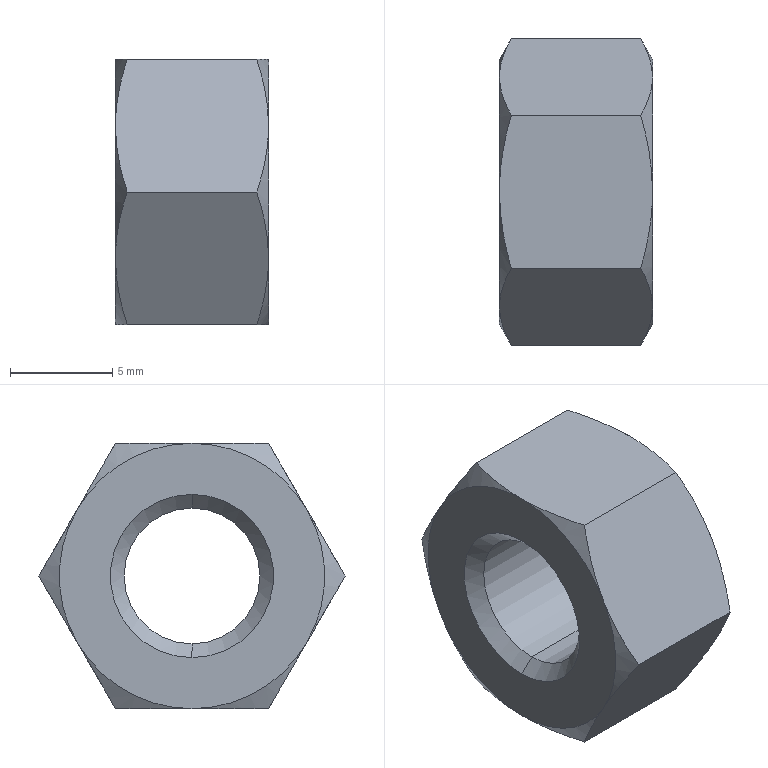Part | STEP file | 001-006-TBK31_M8 | 1 solid | 26 faces | box 7.5 x 15.011 x 13 mm | volume 822.445 mm3 | cone 16 | plane 8 | cylinder 2 | commonest cylinder face diameters 6.647 x2